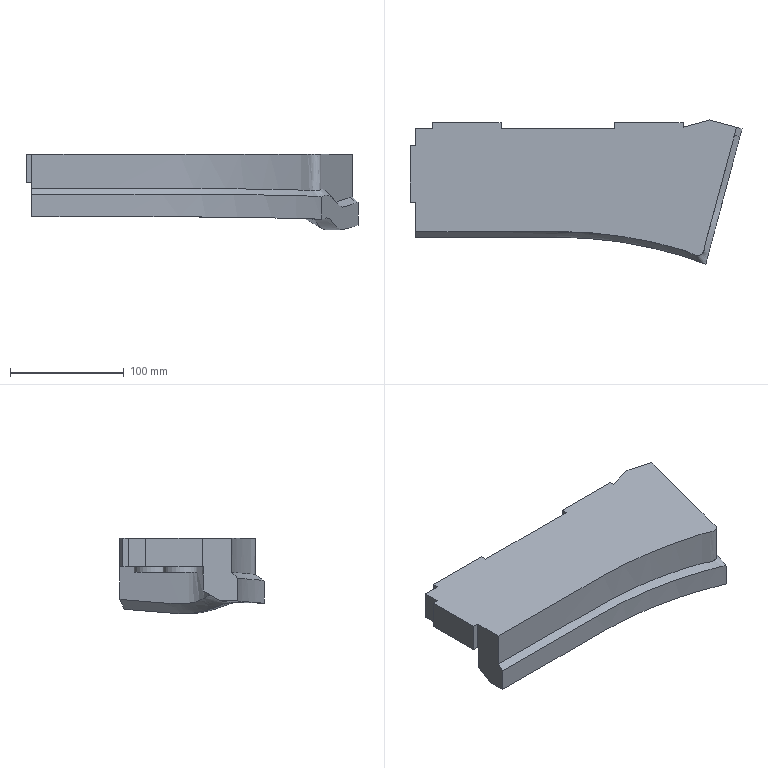Part | NX | features solid 2 | 1 solid | 35 faces | box 292.727 x 126.626 x 66.462 mm | volume 983533 mm3 | plane 23 | spline 7 | cylinder 5 | commonest cylinder face diameters 30 x5